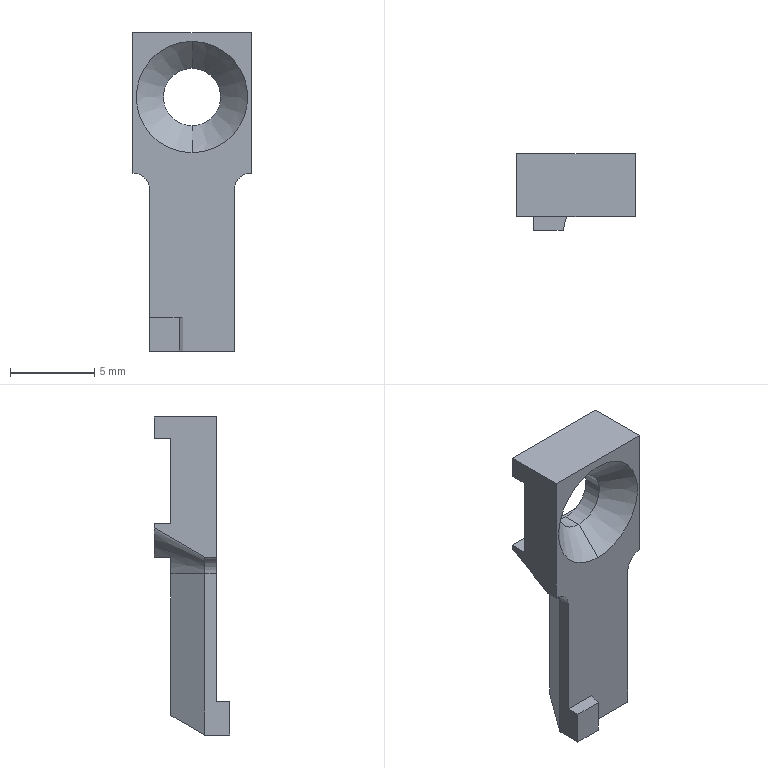Part | SolidWorks | features Cut 5, Chamfer 3, DelFace 1, Extrusion 1, Fillet 1, HoleWzd 1, MoveFace 1 | 1 solid | 26 faces | box 7 x 4.5 x 18.85 mm | volume 263.26 mm3 | plane 19 | cylinder 4 | cone 3 | commonest cylinder face diameters 2 x2 3.4 x2
STEP:
#1=CARTESIAN_POINT('',(0.,-2.1,7.325));
#2=VERTEX_POINT('',#1);
#3=CARTESIAN_POINT('',(0.,-2.1,3.925));
#4=VERTEX_POINT('',#3);
#5=CARTESIAN_POINT('',(0.,-2.1,5.625));
#6=DIRECTION('',(0.,-1.,0.));
#7=DIRECTION('',(0.,0.,-1.));
#8=AXIS2_PLACEMENT_3D('',#5,#6,#7);
#9=CIRCLE('',#8,1.7);
#10=EDGE_CURVE('',#2,#4,#9,.T.);
#11=ORIENTED_EDGE('',*,*,#10,.F.);
#12=CARTESIAN_POINT('',(0.,-3.7,8.925));
#13=VERTEX_POINT('',#12);
#14=CARTESIAN_POINT('',(0.,-3.7,8.925));
#15=DIRECTION('',(0.,-0.7071,0.7071));
#16=VECTOR('',#15,1000.);
#17=LINE('',#14,#16);
#18=EDGE_CURVE('',#2,#13,#17,.T.);
#19=ORIENTED_EDGE('',*,*,#18,.T.);
#20=CARTESIAN_POINT('',(0.,-3.7,2.325));
#21=VERTEX_POINT('',#20);
#22=CARTESIAN_POINT('',(0.,-3.7,5.625));
#23=DIRECTION('',(0.,-1.,0.));
#24=DIRECTION('',(0.,0.,-1.));
#25=AXIS2_PLACEMENT_3D('',#22,#23,#24);
#26=CIRCLE('',#25,3.3);
#27=EDGE_CURVE('',#13,#21,#26,.T.);
#28=ORIENTED_EDGE('',*,*,#27,.T.);
#29=CARTESIAN_POINT('',(0.,-3.7,2.325));
#30=DIRECTION('',(0.,-0.7071,-0.7071));
#31=VECTOR('',#30,1000.);
#32=LINE('',#29,#31);
#33=EDGE_CURVE('',#4,#21,#32,.T.);
#34=ORIENTED_EDGE('',*,*,#33,.F.);
#35=EDGE_LOOP('',(#11,#19,#28,#34));
#36=FACE_OUTER_BOUND('',#35,.T.);
#37=CARTESIAN_POINT('',(0.,-3.7,5.625));
#38=DIRECTION('',(0.,-1.,0.));
#39=DIRECTION('',(0.,0.,-1.));
#40=AXIS2_PLACEMENT_3D('',#37,#38,#39);
#41=CONICAL_SURFACE('',#40,3.3,0.7854);
#42=ADVANCED_FACE('',(#36),#41,.F.);
#43=CARTESIAN_POINT('',(0.,-1.,7.325));
#44=VERTEX_POINT('',#43);
#45=CARTESIAN_POINT('',(0.,-1.,3.925));
#46=VERTEX_POINT('',#45);
#47=CARTESIAN_POINT('',(0.,-1.,5.625));
#48=DIRECTION('',(0.,-1.,0.));
#49=DIRECTION('',(0.,0.,-1.));
#50=AXIS2_PLACEMENT_3D('',#47,#48,#49);
#51=CIRCLE('',#50,1.7);
#52=EDGE_CURVE('',#44,#46,#51,.T.);
#53=ORIENTED_EDGE('',*,*,#52,.F.);
#54=CARTESIAN_POINT('',(0.,-3.7,7.325));
#55=DIRECTION('',(0.,-1.,0.));
#56=VECTOR('',#55,1000.);
#57=LINE('',#54,#56);
#58=EDGE_CURVE('',#44,#2,#57,.T.);
#59=ORIENTED_EDGE('',*,*,#58,.T.);
#60=ORIENTED_EDGE('',*,*,#10,.T.);
#61=CARTESIAN_POINT('',(0.,-3.7,3.925));
#62=DIRECTION('',(0.,-1.,0.));
#63=VECTOR('',#62,1000.);
#64=LINE('',#61,#63);
#65=EDGE_CURVE('',#46,#4,#64,.T.);
#66=ORIENTED_EDGE('',*,*,#65,.F.);
#67=EDGE_LOOP('',(#53,#59,#60,#66));
#68=FACE_OUTER_BOUND('',#67,.T.);
#69=CARTESIAN_POINT('',(0.,-3.7,5.625));
#70=DIRECTION('',(0.,-1.,0.));
#71=DIRECTION('',(0.,0.,-1.));
#72=AXIS2_PLACEMENT_3D('',#69,#70,#71);
#73=CYLINDRICAL_SURFACE('',#72,1.7);
#74=ADVANCED_FACE('',(#68),#73,.F.);
#75=CARTESIAN_POINT('',(-3.5,-3.7,9.425));
#76=VERTEX_POINT('',#75);
#77=CARTESIAN_POINT('',(-3.5,0.,9.425));
#78=VERTEX_POINT('',#77);
#79=CARTESIAN_POINT('',(-3.5,-5.2,9.425));
#80=DIRECTION('',(0.,1.,0.));
#81=VECTOR('',#80,1000.);
#82=LINE('',#79,#81);
#83=EDGE_CURVE('',#76,#78,#82,.T.);
#84=ORIENTED_EDGE('',*,*,#83,.F.);
#85=CARTESIAN_POINT('',(3.5,-3.7,9.425));
#86=VERTEX_POINT('',#85);
#87=CARTESIAN_POINT('',(3.5,-3.7,9.425));
#88=DIRECTION('',(-1.,0.,0.));
#89=VECTOR('',#88,1000.);
#90=LINE('',#87,#89);
#91=EDGE_CURVE('',#86,#76,#90,.T.);
#92=ORIENTED_EDGE('',*,*,#91,.F.);
#93=CARTESIAN_POINT('',(3.5,0.,9.425));
#94=VERTEX_POINT('',#93);
#95=CARTESIAN_POINT('',(3.5,-5.2,9.425));
#96=DIRECTION('',(0.,1.,0.));
#97=VECTOR('',#96,1000.);
#98=LINE('',#95,#97);
#99=EDGE_CURVE('',#86,#94,#98,.T.);
#100=ORIENTED_EDGE('',*,*,#99,.T.);
#101=CARTESIAN_POINT('',(-3.5,0.,9.425));
#102=DIRECTION('',(1.,0.,0.));
#103=VECTOR('',#102,1000.);
#104=LINE('',#101,#103);
#105=EDGE_CURVE('',#78,#94,#104,.T.);
#106=ORIENTED_EDGE('',*,*,#105,.F.);
#107=EDGE_LOOP('',(#84,#92,#100,#106));
#108=FACE_OUTER_BOUND('',#107,.T.);
#109=CARTESIAN_POINT('',(-3.5,-5.2,9.425));
#110=DIRECTION('',(0.,0.,1.));
#111=DIRECTION('',(1.,0.,0.));
#112=AXIS2_PLACEMENT_3D('',#109,#110,#111);
#113=PLANE('',#112);
#114=ADVANCED_FACE('',(#108),#113,.T.);
#115=CARTESIAN_POINT('',(3.5,0.,8.125));
#116=VERTEX_POINT('',#115);
#117=CARTESIAN_POINT('',(3.5,0.,9.425));
#118=DIRECTION('',(0.,0.,-1.));
#119=VECTOR('',#118,1000.);
#120=LINE('',#117,#119);
#121=EDGE_CURVE('',#94,#116,#120,.T.);
#122=ORIENTED_EDGE('',*,*,#121,.T.);
#123=CARTESIAN_POINT('',(-3.5,0.,8.125));
#124=VERTEX_POINT('',#123);
#125=CARTESIAN_POINT('',(-3.5,0.,8.125));
#126=DIRECTION('',(1.,0.,0.));
#127=VECTOR('',#126,1000.);
#128=LINE('',#125,#127);
#129=EDGE_CURVE('',#124,#116,#128,.T.);
#130=ORIENTED_EDGE('',*,*,#129,.F.);
#131=CARTESIAN_POINT('',(-3.5,0.,9.425));
#132=DIRECTION('',(0.,0.,1.));
#133=VECTOR('',#132,1000.);
#134=LINE('',#131,#133);
#135=EDGE_CURVE('',#124,#78,#134,.T.);
#136=ORIENTED_EDGE('',*,*,#135,.T.);
#137=ORIENTED_EDGE('',*,*,#105,.T.);
#138=EDGE_LOOP('',(#122,#130,#136,#137));
#139=FACE_OUTER_BOUND('',#138,.T.);
#140=CARTESIAN_POINT('',(0.,0.,0.));
#141=DIRECTION('',(0.,-1.,0.));
#142=DIRECTION('',(0.,0.,-1.));
#143=AXIS2_PLACEMENT_3D('',#140,#141,#142);
#144=PLANE('',#143);
#145=ADVANCED_FACE('',(#139),#144,.F.);
#146=CARTESIAN_POINT('',(3.5,-3.7,1.125));
#147=VERTEX_POINT('',#146);
#148=CARTESIAN_POINT('',(3.5,-3.7,-7.425));
#149=DIRECTION('',(0.,0.,1.));
#150=VECTOR('',#149,1000.);
#151=LINE('',#148,#150);
#152=EDGE_CURVE('',#147,#86,#151,.T.);
#153=ORIENTED_EDGE('',*,*,#152,.F.);
#154=CARTESIAN_POINT('',(3.5,-1.,1.125));
#155=VERTEX_POINT('',#154);
#156=CARTESIAN_POINT('',(3.5,0.,1.125));
#157=DIRECTION('',(0.,-1.,0.));
#158=VECTOR('',#157,1000.);
#159=LINE('',#156,#158);
#160=EDGE_CURVE('',#155,#147,#159,.T.);
#161=ORIENTED_EDGE('',*,*,#160,.F.);
#162=CARTESIAN_POINT('',(3.5,0.,1.125));
#163=VERTEX_POINT('',#162);
#164=CARTESIAN_POINT('',(3.5,0.,1.125));
#165=DIRECTION('',(0.,-1.,0.));
#166=VECTOR('',#165,1000.);
#167=LINE('',#164,#166);
#168=EDGE_CURVE('',#163,#155,#167,.T.);
#169=ORIENTED_EDGE('',*,*,#168,.F.);
#170=CARTESIAN_POINT('',(3.5,0.,3.125));
#171=VERTEX_POINT('',#170);
#172=CARTESIAN_POINT('',(3.5,0.,9.425));
#173=DIRECTION('',(0.,0.,-1.));
#174=VECTOR('',#173,1000.);
#175=LINE('',#172,#174);
#176=EDGE_CURVE('',#171,#163,#175,.T.);
#177=ORIENTED_EDGE('',*,*,#176,.F.);
#178=CARTESIAN_POINT('',(3.5,-1.,3.125));
#179=VERTEX_POINT('',#178);
#180=CARTESIAN_POINT('',(3.5,0.,3.125));
#181=DIRECTION('',(0.,1.,0.));
#182=VECTOR('',#181,1000.);
#183=LINE('',#180,#182);
#184=EDGE_CURVE('',#179,#171,#183,.T.);
#185=ORIENTED_EDGE('',*,*,#184,.F.);
#186=CARTESIAN_POINT('',(3.5,-1.,8.125));
#187=VERTEX_POINT('',#186);
#188=CARTESIAN_POINT('',(3.5,-1.,8.125));
#189=DIRECTION('',(0.,0.,-1.));
#190=VECTOR('',#189,1000.);
#191=LINE('',#188,#190);
#192=EDGE_CURVE('',#187,#179,#191,.T.);
#193=ORIENTED_EDGE('',*,*,#192,.F.);
#194=CARTESIAN_POINT('',(3.5,0.,8.125));
#195=DIRECTION('',(0.,-1.,0.));
#196=VECTOR('',#195,1000.);
#197=LINE('',#194,#196);
#198=EDGE_CURVE('',#116,#187,#197,.T.);
#199=ORIENTED_EDGE('',*,*,#198,.F.);
#200=ORIENTED_EDGE('',*,*,#121,.F.);
#201=ORIENTED_EDGE('',*,*,#99,.F.);
#202=EDGE_LOOP('',(#153,#161,#169,#177,#185,#193,#199,#200,#201));
#203=FACE_OUTER_BOUND('',#202,.T.);
#204=CARTESIAN_POINT('',(3.5,-5.2,9.425));
#205=DIRECTION('',(1.,0.,0.));
#206=DIRECTION('',(0.,0.,-1.));
#207=AXIS2_PLACEMENT_3D('',#204,#205,#206);
#208=PLANE('',#207);
#209=ADVANCED_FACE('',(#203),#208,.T.);
#210=CARTESIAN_POINT('',(-3.5,0.,2.857));
#211=VERTEX_POINT('',#210);
#212=CARTESIAN_POINT('',(-3.5,0.,3.125));
#213=VERTEX_POINT('',#212);
#214=CARTESIAN_POINT('',(-3.5,0.,9.425));
#215=DIRECTION('',(0.,0.,1.));
#216=VECTOR('',#215,1000.);
#217=LINE('',#214,#216);
#218=EDGE_CURVE('',#211,#213,#217,.T.);
#219=ORIENTED_EDGE('',*,*,#218,.F.);
#220=CARTESIAN_POINT('',(-3.5,-3.,1.125));
#221=VERTEX_POINT('',#220);
#222=CARTESIAN_POINT('',(-3.5,-4.732,0.125));
#223=DIRECTION('',(0.,-0.866,-0.5));
#224=VECTOR('',#223,1000.);
#225=LINE('',#222,#224);
#226=EDGE_CURVE('',#211,#221,#225,.T.);
#227=ORIENTED_EDGE('',*,*,#226,.T.);
#228=CARTESIAN_POINT('',(-3.5,-3.7,1.125));
#229=VERTEX_POINT('',#228);
#230=CARTESIAN_POINT('',(-3.5,0.,1.125));
#231=DIRECTION('',(0.,-1.,0.));
#232=VECTOR('',#231,1000.);
#233=LINE('',#230,#232);
#234=EDGE_CURVE('',#221,#229,#233,.T.);
#235=ORIENTED_EDGE('',*,*,#234,.T.);
#236=CARTESIAN_POINT('',(-3.5,-3.7,9.425));
#237=DIRECTION('',(0.,0.,-1.));
#238=VECTOR('',#237,1000.);
#239=LINE('',#236,#238);
#240=EDGE_CURVE('',#76,#229,#239,.T.);
#241=ORIENTED_EDGE('',*,*,#240,.F.);
#242=ORIENTED_EDGE('',*,*,#83,.T.);
#243=ORIENTED_EDGE('',*,*,#135,.F.);
#244=CARTESIAN_POINT('',(-3.5,-1.,8.125));
#245=VERTEX_POINT('',#244);
#246=CARTESIAN_POINT('',(-3.5,0.,8.125));
#247=DIRECTION('',(0.,-1.,0.));
#248=VECTOR('',#247,1000.);
#249=LINE('',#246,#248);
#250=EDGE_CURVE('',#124,#245,#249,.T.);
#251=ORIENTED_EDGE('',*,*,#250,.T.);
#252=CARTESIAN_POINT('',(-3.5,-1.,3.125));
#253=VERTEX_POINT('',#252);
#254=CARTESIAN_POINT('',(-3.5,-1.,8.125));
#255=DIRECTION('',(0.,0.,-1.));
#256=VECTOR('',#255,1000.);
#257=LINE('',#254,#256);
#258=EDGE_CURVE('',#245,#253,#257,.T.);
#259=ORIENTED_EDGE('',*,*,#258,.T.);
#260=CARTESIAN_POINT('',(-3.5,0.,3.125));
#261=DIRECTION('',(0.,1.,0.));
#262=VECTOR('',#261,1000.);
#263=LINE('',#260,#262);
#264=EDGE_CURVE('',#253,#213,#263,.T.);
#265=ORIENTED_EDGE('',*,*,#264,.T.);
#266=EDGE_LOOP('',(#219,#227,#235,#241,#242,#243,#251,#259,#265));
#267=FACE_OUTER_BOUND('',#266,.T.);
#268=CARTESIAN_POINT('',(-3.5,-5.2,9.425));
#269=DIRECTION('',(-1.,0.,0.));
#270=DIRECTION('',(0.,0.,1.));
#271=AXIS2_PLACEMENT_3D('',#268,#269,#270);
#272=PLANE('',#271);
#273=ADVANCED_FACE('',(#267),#272,.T.);
#274=CARTESIAN_POINT('',(-2.5,-4.5,-9.425));
#275=VERTEX_POINT('',#274);
#276=CARTESIAN_POINT('',(-2.5,-3.,-9.425));
#277=VERTEX_POINT('',#276);
#278=CARTESIAN_POINT('',(-2.5,-5.2,-9.425));
#279=DIRECTION('',(0.,1.,0.));
#280=VECTOR('',#279,1000.);
#281=LINE('',#278,#280);
#282=EDGE_CURVE('',#275,#277,#281,.T.);
#283=ORIENTED_EDGE('',*,*,#282,.T.);
#284=CARTESIAN_POINT('',(2.5,-3.,-9.425));
#285=VERTEX_POINT('',#284);
#286=CARTESIAN_POINT('',(2.5,-3.,-9.425));
#287=DIRECTION('',(1.,0.,0.));
#288=VECTOR('',#287,1000.);
#289=LINE('',#286,#288);
#290=EDGE_CURVE('',#277,#285,#289,.T.);
#291=ORIENTED_EDGE('',*,*,#290,.T.);
#292=CARTESIAN_POINT('',(2.5,-3.7,-9.425));
#293=VERTEX_POINT('',#292);
#294=CARTESIAN_POINT('',(2.5,-5.2,-9.425));
#295=DIRECTION('',(0.,1.,0.));
#296=VECTOR('',#295,1000.);
#297=LINE('',#294,#296);
#298=EDGE_CURVE('',#293,#285,#297,.T.);
#299=ORIENTED_EDGE('',*,*,#298,.F.);
#300=CARTESIAN_POINT('',(-0.5536,-3.7,-9.425));
#301=VERTEX_POINT('',#300);
#302=CARTESIAN_POINT('',(-0.5,-3.7,-9.425));
#303=DIRECTION('',(1.,0.,0.));
#304=VECTOR('',#303,1000.);
#305=LINE('',#302,#304);
#306=EDGE_CURVE('',#301,#293,#305,.T.);
#307=ORIENTED_EDGE('',*,*,#306,.F.);
#308=CARTESIAN_POINT('',(-0.7679,-4.5,-9.425));
#309=VERTEX_POINT('',#308);
#310=CARTESIAN_POINT('',(-0.951,-5.183,-9.425));
#311=DIRECTION('',(-0.2588,-0.9659,0.));
#312=VECTOR('',#311,1000.);
#313=LINE('',#310,#312);
#314=EDGE_CURVE('',#301,#309,#313,.T.);
#315=ORIENTED_EDGE('',*,*,#314,.T.);
#316=CARTESIAN_POINT('',(-3.5,-4.5,-9.425));
#317=DIRECTION('',(-1.,0.,0.));
#318=VECTOR('',#317,1000.);
#319=LINE('',#316,#318);
#320=EDGE_CURVE('',#309,#275,#319,.T.);
#321=ORIENTED_EDGE('',*,*,#320,.T.);
#322=EDGE_LOOP('',(#283,#291,#299,#307,#315,#321));
#323=FACE_OUTER_BOUND('',#322,.T.);
#324=CARTESIAN_POINT('',(-3.5,-5.2,-9.425));
#325=DIRECTION('',(0.,0.,-1.));
#326=DIRECTION('',(-1.,0.,0.));
#327=AXIS2_PLACEMENT_3D('',#324,#325,#326);
#328=PLANE('',#327);
#329=ADVANCED_FACE('',(#323),#328,.T.);
#330=ORIENTED_EDGE('',*,*,#320,.F.);
#331=CARTESIAN_POINT('',(-0.7679,-4.5,-7.425));
#332=VERTEX_POINT('',#331);
#333=CARTESIAN_POINT('',(-0.7679,-4.5,-8.085));
#334=DIRECTION('',(0.,0.,1.));
#335=VECTOR('',#334,1000.);
#336=LINE('',#333,#335);
#337=EDGE_CURVE('',#309,#332,#336,.T.);
#338=ORIENTED_EDGE('',*,*,#337,.T.);
#339=CARTESIAN_POINT('',(-2.5,-4.5,-7.425));
#340=VERTEX_POINT('',#339);
#341=CARTESIAN_POINT('',(-3.5,-4.5,-7.425));
#342=DIRECTION('',(1.,0.,0.));
#343=VECTOR('',#342,1000.);
#344=LINE('',#341,#343);
#345=EDGE_CURVE('',#340,#332,#344,.T.);
#346=ORIENTED_EDGE('',*,*,#345,.F.);
#347=CARTESIAN_POINT('',(-2.5,-4.5,-9.425));
#348=DIRECTION('',(0.,0.,-1.));
#349=VECTOR('',#348,1000.);
#350=LINE('',#347,#349);
#351=EDGE_CURVE('',#340,#275,#350,.T.);
#352=ORIENTED_EDGE('',*,*,#351,.T.);
#353=EDGE_LOOP('',(#330,#338,#346,#352));
#354=FACE_OUTER_BOUND('',#353,.T.);
#355=CARTESIAN_POINT('',(0.,-4.5,0.));
#356=DIRECTION('',(0.,-1.,0.));
#357=DIRECTION('',(0.,0.,-1.));
#358=AXIS2_PLACEMENT_3D('',#355,#356,#357);
#359=PLANE('',#358);
#360=ADVANCED_FACE('',(#354),#359,.T.);
#361=CARTESIAN_POINT('',(-0.9575,0.,1.125));
#362=VERTEX_POINT('',#361);
#363=CARTESIAN_POINT('',(-3.5,0.,1.125));
#364=DIRECTION('',(1.,0.,0.));
#365=VECTOR('',#364,1000.);
#366=LINE('',#363,#365);
#367=EDGE_CURVE('',#362,#163,#366,.T.);
#368=ORIENTED_EDGE('',*,*,#367,.F.);
#369=CARTESIAN_POINT('',(-3.5,0.,0.125));
#370=DIRECTION('',(0.,-1.,0.));
#371=DIRECTION('',(0.,0.,-1.));
#372=AXIS2_PLACEMENT_3D('',#369,#370,#371);
#373=CIRCLE('',#372,2.732);
#374=EDGE_CURVE('',#362,#211,#373,.T.);
#375=ORIENTED_EDGE('',*,*,#374,.T.);
#376=ORIENTED_EDGE('',*,*,#218,.T.);
#377=CARTESIAN_POINT('',(-3.5,0.,3.125));
#378=DIRECTION('',(1.,0.,0.));
#379=VECTOR('',#378,1000.);
#380=LINE('',#377,#379);
#381=EDGE_CURVE('',#213,#171,#380,.T.);
#382=ORIENTED_EDGE('',*,*,#381,.T.);
#383=ORIENTED_EDGE('',*,*,#176,.T.);
#384=EDGE_LOOP('',(#368,#375,#376,#382,#383));
#385=FACE_OUTER_BOUND('',#384,.T.);
#386=CARTESIAN_POINT('',(0.,0.,0.));
#387=DIRECTION('',(0.,-1.,0.));
#388=DIRECTION('',(0.,0.,-1.));
#389=AXIS2_PLACEMENT_3D('',#386,#387,#388);
#390=PLANE('',#389);
#391=ADVANCED_FACE('',(#385),#390,.F.);
#392=ORIENTED_EDGE('',*,*,#198,.T.);
#393=CARTESIAN_POINT('',(-3.5,-1.,8.125));
#394=DIRECTION('',(1.,0.,0.));
#395=VECTOR('',#394,1000.);
#396=LINE('',#393,#395);
#397=EDGE_CURVE('',#245,#187,#396,.T.);
#398=ORIENTED_EDGE('',*,*,#397,.F.);
#399=ORIENTED_EDGE('',*,*,#250,.F.);
#400=ORIENTED_EDGE('',*,*,#129,.T.);
#401=EDGE_LOOP('',(#392,#398,#399,#400));
#402=FACE_OUTER_BOUND('',#401,.T.);
#403=CARTESIAN_POINT('',(-3.5,0.,8.125));
#404=DIRECTION('',(0.,0.,1.));
#405=DIRECTION('',(1.,0.,0.));
#406=AXIS2_PLACEMENT_3D('',#403,#404,#405);
#407=PLANE('',#406);
#408=ADVANCED_FACE('',(#402),#407,.F.);
#409=ORIENTED_EDGE('',*,*,#184,.T.);
#410=ORIENTED_EDGE('',*,*,#381,.F.);
#411=ORIENTED_EDGE('',*,*,#264,.F.);
#412=CARTESIAN_POINT('',(-3.5,-1.,3.125));
#413=DIRECTION('',(1.,0.,0.));
#414=VECTOR('',#413,1000.);
#415=LINE('',#412,#414);
#416=EDGE_CURVE('',#253,#179,#415,.T.);
#417=ORIENTED_EDGE('',*,*,#416,.T.);
#418=EDGE_LOOP('',(#409,#410,#411,#417));
#419=FACE_OUTER_BOUND('',#418,.T.);
#420=CARTESIAN_POINT('',(-3.5,0.,3.125));
#421=DIRECTION('',(0.,0.,-1.));
#422=DIRECTION('',(-1.,0.,0.));
#423=AXIS2_PLACEMENT_3D('',#420,#421,#422);
#424=PLANE('',#423);
#425=ADVANCED_FACE('',(#419),#424,.F.);
#426=CARTESIAN_POINT('',(0.,-1.,5.625));
#427=DIRECTION('',(0.,-1.,0.));
#428=DIRECTION('',(0.,0.,-1.));
#429=AXIS2_PLACEMENT_3D('',#426,#427,#428);
#430=CIRCLE('',#429,1.7);
#431=EDGE_CURVE('',#46,#44,#430,.T.);
#432=ORIENTED_EDGE('',*,*,#431,.T.);
#433=ORIENTED_EDGE('',*,*,#52,.T.);
#434=EDGE_LOOP('',(#432,#433));
#435=FACE_BOUND('',#434,.T.);
#436=ORIENTED_EDGE('',*,*,#192,.T.);
#437=ORIENTED_EDGE('',*,*,#416,.F.);
#438=ORIENTED_EDGE('',*,*,#258,.F.);
#439=ORIENTED_EDGE('',*,*,#397,.T.);
#440=EDGE_LOOP('',(#436,#437,#438,#439));
#441=FACE_OUTER_BOUND('',#440,.T.);
#442=CARTESIAN_POINT('',(-3.5,-1.,8.125));
#443=DIRECTION('',(0.,-1.,0.));
#444=DIRECTION('',(0.,0.,-1.));
#445=AXIS2_PLACEMENT_3D('',#442,#443,#444);
#446=PLANE('',#445);
#447=ADVANCED_FACE('',(#435,#441),#446,.F.);
#448=CARTESIAN_POINT('',(-1.591,-1.,1.125));
#449=VERTEX_POINT('',#448);
#450=CARTESIAN_POINT('',(-3.5,-1.,1.125));
#451=DIRECTION('',(1.,0.,0.));
#452=VECTOR('',#451,1000.);
#453=LINE('',#450,#452);
#454=EDGE_CURVE('',#449,#155,#453,.T.);
#455=ORIENTED_EDGE('',*,*,#454,.F.);
#456=CARTESIAN_POINT('',(-1.591,-1.,1.125));
#457=CARTESIAN_POINT('',(-1.376,-0.6693,1.125));
#458=CARTESIAN_POINT('',(-1.166,-0.3354,1.125));
#459=CARTESIAN_POINT('',(-0.9575,0.,1.125));
#460=B_SPLINE_CURVE_WITH_KNOTS('',3,(#456,#457,#458,#459),.UNSPECIFIED.,.F.,.F.,(4,4),(0.,0.001184),.UNSPECIFIED.);
#461=EDGE_CURVE('',#449,#362,#460,.T.);
#462=ORIENTED_EDGE('',*,*,#461,.T.);
#463=ORIENTED_EDGE('',*,*,#367,.T.);
#464=ORIENTED_EDGE('',*,*,#168,.T.);
#465=EDGE_LOOP('',(#455,#462,#463,#464));
#466=FACE_OUTER_BOUND('',#465,.T.);
#467=CARTESIAN_POINT('',(-3.5,0.,1.125));
#468=DIRECTION('',(0.,0.,1.));
#469=DIRECTION('',(0.,-1.,0.));
#470=AXIS2_PLACEMENT_3D('',#467,#468,#469);
#471=PLANE('',#470);
#472=ADVANCED_FACE('',(#466),#471,.F.);
#473=CARTESIAN_POINT('',(-1.345,-1.,-8.27));
#474=VERTEX_POINT('',#473);
#475=CARTESIAN_POINT('',(-1.345,-1.,0.125));
#476=VERTEX_POINT('',#475);
#477=CARTESIAN_POINT('',(-1.345,-1.,1.125));
#478=DIRECTION('',(0.,0.,1.));
#479=VECTOR('',#478,1000.);
#480=LINE('',#477,#479);
#481=EDGE_CURVE('',#474,#476,#480,.T.);
#482=ORIENTED_EDGE('',*,*,#481,.T.);
#483=CARTESIAN_POINT('',(-3.5,-1.,0.125));
#484=DIRECTION('',(0.,-1.,0.));
#485=DIRECTION('',(0.,0.,-1.));
#486=AXIS2_PLACEMENT_3D('',#483,#484,#485);
#487=CIRCLE('',#486,2.155);
#488=EDGE_CURVE('',#476,#449,#487,.T.);
#489=ORIENTED_EDGE('',*,*,#488,.T.);
#490=ORIENTED_EDGE('',*,*,#454,.T.);
#491=CARTESIAN_POINT('',(2.5,-1.,0.125));
#492=VERTEX_POINT('',#491);
#493=CARTESIAN_POINT('',(3.5,-1.,0.125));
#494=DIRECTION('',(0.,-1.,0.));
#495=DIRECTION('',(0.,0.,-1.));
#496=AXIS2_PLACEMENT_3D('',#493,#494,#495);
#497=CIRCLE('',#496,1.);
#498=EDGE_CURVE('',#155,#492,#497,.T.);
#499=ORIENTED_EDGE('',*,*,#498,.T.);
#500=CARTESIAN_POINT('',(2.5,-1.,-8.27));
#501=VERTEX_POINT('',#500);
#502=CARTESIAN_POINT('',(2.5,-1.,-9.425));
#503=DIRECTION('',(0.,0.,1.));
#504=VECTOR('',#503,1000.);
#505=LINE('',#502,#504);
#506=EDGE_CURVE('',#501,#492,#505,.T.);
#507=ORIENTED_EDGE('',*,*,#506,.F.);
#508=CARTESIAN_POINT('',(-2.5,-1.,-8.27));
#509=DIRECTION('',(-1.,0.,0.));
#510=VECTOR('',#509,1000.);
#511=LINE('',#508,#510);
#512=EDGE_CURVE('',#501,#474,#511,.T.);
#513=ORIENTED_EDGE('',*,*,#512,.T.);
#514=EDGE_LOOP('',(#482,#489,#490,#499,#507,#513));
#515=FACE_OUTER_BOUND('',#514,.T.);
#516=CARTESIAN_POINT('',(-3.5,-1.,1.125));
#517=DIRECTION('',(0.,-1.,0.));
#518=DIRECTION('',(0.,0.,-1.));
#519=AXIS2_PLACEMENT_3D('',#516,#517,#518);
#520=PLANE('',#519);
#521=ADVANCED_FACE('',(#515),#520,.F.);
#522=CARTESIAN_POINT('',(-0.5536,-3.7,-7.425));
#523=VERTEX_POINT('',#522);
#524=CARTESIAN_POINT('',(-0.5,-3.5,-7.425));
#525=DIRECTION('',(0.2588,0.9659,0.));
#526=VECTOR('',#525,1000.);
#527=LINE('',#524,#526);
#528=EDGE_CURVE('',#332,#523,#527,.T.);
#529=ORIENTED_EDGE('',*,*,#528,.T.);
#530=CARTESIAN_POINT('',(-2.5,-3.7,-7.425));
#531=VERTEX_POINT('',#530);
#532=CARTESIAN_POINT('',(0.48,-3.7,-7.425));
#533=DIRECTION('',(1.,0.,0.));
#534=VECTOR('',#533,1000.);
#535=LINE('',#532,#534);
#536=EDGE_CURVE('',#531,#523,#535,.T.);
#537=ORIENTED_EDGE('',*,*,#536,.F.);
#538=CARTESIAN_POINT('',(-2.5,-3.7,-7.425));
#539=DIRECTION('',(0.,-1.,0.));
#540=VECTOR('',#539,1000.);
#541=LINE('',#538,#540);
#542=EDGE_CURVE('',#531,#340,#541,.T.);
#543=ORIENTED_EDGE('',*,*,#542,.T.);
#544=ORIENTED_EDGE('',*,*,#345,.T.);
#545=EDGE_LOOP('',(#529,#537,#543,#544));
#546=FACE_OUTER_BOUND('',#545,.T.);
#547=CARTESIAN_POINT('',(0.48,-3.7,-7.425));
#548=DIRECTION('',(0.,0.,-1.));
#549=DIRECTION('',(-1.,0.,0.));
#550=AXIS2_PLACEMENT_3D('',#547,#548,#549);
#551=PLANE('',#550);
#552=ADVANCED_FACE('',(#546),#551,.F.);
#553=CARTESIAN_POINT('',(0.,-3.7,5.625));
#554=DIRECTION('',(0.,-1.,0.));
#555=DIRECTION('',(0.,0.,-1.));
#556=AXIS2_PLACEMENT_3D('',#553,#554,#555);
#557=CIRCLE('',#556,3.3);
#558=EDGE_CURVE('',#21,#13,#557,.T.);
#559=ORIENTED_EDGE('',*,*,#558,.F.);
#560=ORIENTED_EDGE('',*,*,#27,.F.);
#561=EDGE_LOOP('',(#559,#560));
#562=FACE_BOUND('',#561,.T.);
#563=CARTESIAN_POINT('',(2.5,-3.7,0.125));
#564=VERTEX_POINT('',#563);
#565=CARTESIAN_POINT('',(2.5,-3.7,-6.345));
#566=DIRECTION('',(0.,0.,-1.));
#567=VECTOR('',#566,1000.);
#568=LINE('',#565,#567);
#569=EDGE_CURVE('',#564,#293,#568,.T.);
#570=ORIENTED_EDGE('',*,*,#569,.F.);
#571=CARTESIAN_POINT('',(3.5,-3.7,0.125));
#572=DIRECTION('',(0.,1.,0.));
#573=DIRECTION('',(0.,0.,-1.));
#574=AXIS2_PLACEMENT_3D('',#571,#572,#573);
#575=CIRCLE('',#574,1.);
#576=EDGE_CURVE('',#564,#147,#575,.T.);
#577=ORIENTED_EDGE('',*,*,#576,.T.);
#578=ORIENTED_EDGE('',*,*,#152,.T.);
#579=ORIENTED_EDGE('',*,*,#91,.T.);
#580=ORIENTED_EDGE('',*,*,#240,.T.);
#581=CARTESIAN_POINT('',(-2.5,-3.7,0.125));
#582=VERTEX_POINT('',#581);
#583=CARTESIAN_POINT('',(-3.5,-3.7,0.125));
#584=DIRECTION('',(0.,1.,0.));
#585=DIRECTION('',(0.,0.,-1.));
#586=AXIS2_PLACEMENT_3D('',#583,#584,#585);
#587=CIRCLE('',#586,1.);
#588=EDGE_CURVE('',#229,#582,#587,.T.);
#589=ORIENTED_EDGE('',*,*,#588,.T.);
#590=CARTESIAN_POINT('',(-2.5,-3.7,-6.345));
#591=DIRECTION('',(0.,0.,1.));
#592=VECTOR('',#591,1000.);
#593=LINE('',#590,#592);
#594=EDGE_CURVE('',#531,#582,#593,.T.);
#595=ORIENTED_EDGE('',*,*,#594,.F.);
#596=ORIENTED_EDGE('',*,*,#536,.T.);
#597=CARTESIAN_POINT('',(-0.5536,-3.7,9.425));
#598=DIRECTION('',(0.,0.,-1.));
#599=VECTOR('',#598,1000.);
#600=LINE('',#597,#599);
#601=EDGE_CURVE('',#523,#301,#600,.T.);
#602=ORIENTED_EDGE('',*,*,#601,.T.);
#603=ORIENTED_EDGE('',*,*,#306,.T.);
#604=EDGE_LOOP('',(#570,#577,#578,#579,#580,#589,#595,#596,#602,#603));
#605=FACE_OUTER_BOUND('',#604,.T.);
#606=CARTESIAN_POINT('',(-0.96,-3.7,-6.345));
#607=DIRECTION('',(0.,-1.,0.));
#608=DIRECTION('',(0.,0.,-1.));
#609=AXIS2_PLACEMENT_3D('',#606,#607,#608);
#610=PLANE('',#609);
#611=ADVANCED_FACE('',(#562,#605),#610,.T.);
#612=CARTESIAN_POINT('',(-2.5,-3.,0.125));
#613=VERTEX_POINT('',#612);
#614=CARTESIAN_POINT('',(-2.5,-1.,0.125));
#615=DIRECTION('',(0.,1.,0.));
#616=VECTOR('',#615,1000.);
#617=LINE('',#614,#616);
#618=EDGE_CURVE('',#582,#613,#617,.T.);
#619=ORIENTED_EDGE('',*,*,#618,.T.);
#620=CARTESIAN_POINT('',(-2.5,-3.,-9.425));
#621=DIRECTION('',(0.,0.,-1.));
#622=VECTOR('',#621,1000.);
#623=LINE('',#620,#622);
#624=EDGE_CURVE('',#613,#277,#623,.T.);
#625=ORIENTED_EDGE('',*,*,#624,.T.);
#626=ORIENTED_EDGE('',*,*,#282,.F.);
#627=ORIENTED_EDGE('',*,*,#351,.F.);
#628=ORIENTED_EDGE('',*,*,#542,.F.);
#629=ORIENTED_EDGE('',*,*,#594,.T.);
#630=EDGE_LOOP('',(#619,#625,#626,#627,#628,#629));
#631=FACE_OUTER_BOUND('',#630,.T.);
#632=CARTESIAN_POINT('',(-2.5,-5.2,-9.425));
#633=DIRECTION('',(1.,0.,0.));
#634=DIRECTION('',(0.,0.,-1.));
#635=AXIS2_PLACEMENT_3D('',#632,#633,#634);
#636=PLANE('',#635);
#637=ADVANCED_FACE('',(#631),#636,.F.);
#638=ORIENTED_EDGE('',*,*,#298,.T.);
#639=CARTESIAN_POINT('',(2.5,-3.,-9.425));
#640=DIRECTION('',(0.,0.866,0.5));
#641=VECTOR('',#640,1000.);
#642=LINE('',#639,#641);
#643=EDGE_CURVE('',#285,#501,#642,.T.);
#644=ORIENTED_EDGE('',*,*,#643,.T.);
#645=ORIENTED_EDGE('',*,*,#506,.T.);
#646=CARTESIAN_POINT('',(2.5,-3.7,0.125));
#647=DIRECTION('',(0.,-1.,0.));
#648=VECTOR('',#647,1000.);
#649=LINE('',#646,#648);
#650=EDGE_CURVE('',#492,#564,#649,.T.);
#651=ORIENTED_EDGE('',*,*,#650,.T.);
#652=ORIENTED_EDGE('',*,*,#569,.T.);
#653=EDGE_LOOP('',(#638,#644,#645,#651,#652));
#654=FACE_OUTER_BOUND('',#653,.T.);
#655=CARTESIAN_POINT('',(2.5,-5.2,-9.425));
#656=DIRECTION('',(-1.,0.,0.));
#657=DIRECTION('',(0.,0.,1.));
#658=AXIS2_PLACEMENT_3D('',#655,#656,#657);
#659=PLANE('',#658);
#660=ADVANCED_FACE('',(#654),#659,.F.);
#661=ORIENTED_EDGE('',*,*,#58,.F.);
#662=ORIENTED_EDGE('',*,*,#431,.F.);
#663=ORIENTED_EDGE('',*,*,#65,.T.);
#664=CARTESIAN_POINT('',(0.,-2.1,5.625));
#665=DIRECTION('',(0.,-1.,0.));
#666=DIRECTION('',(0.,0.,-1.));
#667=AXIS2_PLACEMENT_3D('',#664,#665,#666);
#668=CIRCLE('',#667,1.7);
#669=EDGE_CURVE('',#4,#2,#668,.T.);
#670=ORIENTED_EDGE('',*,*,#669,.T.);
#671=EDGE_LOOP('',(#661,#662,#663,#670));
#672=FACE_OUTER_BOUND('',#671,.T.);
#673=CARTESIAN_POINT('',(0.,-3.7,5.625));
#674=DIRECTION('',(0.,-1.,0.));
#675=DIRECTION('',(0.,0.,-1.));
#676=AXIS2_PLACEMENT_3D('',#673,#674,#675);
#677=CYLINDRICAL_SURFACE('',#676,1.7);
#678=ADVANCED_FACE('',(#672),#677,.F.);
#679=ORIENTED_EDGE('',*,*,#18,.F.);
#680=ORIENTED_EDGE('',*,*,#669,.F.);
#681=ORIENTED_EDGE('',*,*,#33,.T.);
#682=ORIENTED_EDGE('',*,*,#558,.T.);
#683=EDGE_LOOP('',(#679,#680,#681,#682));
#684=FACE_OUTER_BOUND('',#683,.T.);
#685=CARTESIAN_POINT('',(0.,-3.7,5.625));
#686=DIRECTION('',(0.,-1.,0.));
#687=DIRECTION('',(0.,0.,-1.));
#688=AXIS2_PLACEMENT_3D('',#685,#686,#687);
#689=CONICAL_SURFACE('',#688,3.3,0.7854);
#690=ADVANCED_FACE('',(#684),#689,.F.);
#691=ORIENTED_EDGE('',*,*,#234,.F.);
#692=CARTESIAN_POINT('',(-3.5,-3.,0.125));
#693=DIRECTION('',(0.,1.,0.));
#694=DIRECTION('',(0.,0.,-1.));
#695=AXIS2_PLACEMENT_3D('',#692,#693,#694);
#696=CIRCLE('',#695,1.);
#697=EDGE_CURVE('',#221,#613,#696,.T.);
#698=ORIENTED_EDGE('',*,*,#697,.T.);
#699=ORIENTED_EDGE('',*,*,#618,.F.);
#700=ORIENTED_EDGE('',*,*,#588,.F.);
#701=EDGE_LOOP('',(#691,#698,#699,#700));
#702=FACE_OUTER_BOUND('',#701,.T.);
#703=CARTESIAN_POINT('',(-3.5,-5.2,0.125));
#704=DIRECTION('',(0.,-1.,0.));
#705=DIRECTION('',(0.,0.,-1.));
#706=AXIS2_PLACEMENT_3D('',#703,#704,#705);
#707=CYLINDRICAL_SURFACE('',#706,1.);
#708=ADVANCED_FACE('',(#702),#707,.F.);
#709=ORIENTED_EDGE('',*,*,#576,.F.);
#710=ORIENTED_EDGE('',*,*,#650,.F.);
#711=ORIENTED_EDGE('',*,*,#498,.F.);
#712=ORIENTED_EDGE('',*,*,#160,.T.);
#713=EDGE_LOOP('',(#709,#710,#711,#712));
#714=FACE_OUTER_BOUND('',#713,.T.);
#715=CARTESIAN_POINT('',(3.5,0.,0.125));
#716=DIRECTION('',(0.,-1.,0.));
#717=DIRECTION('',(0.,0.,-1.));
#718=AXIS2_PLACEMENT_3D('',#715,#716,#717);
#719=CYLINDRICAL_SURFACE('',#718,1.);
#720=ADVANCED_FACE('',(#714),#719,.F.);
#721=ORIENTED_EDGE('',*,*,#601,.F.);
#722=ORIENTED_EDGE('',*,*,#528,.F.);
#723=ORIENTED_EDGE('',*,*,#337,.F.);
#724=ORIENTED_EDGE('',*,*,#314,.F.);
#725=EDGE_LOOP('',(#721,#722,#723,#724));
#726=FACE_OUTER_BOUND('',#725,.T.);
#727=CARTESIAN_POINT('',(-0.5,-3.5,9.425));
#728=DIRECTION('',(0.9659,-0.2588,0.));
#729=DIRECTION('',(0.,0.,1.));
#730=AXIS2_PLACEMENT_3D('',#727,#728,#729);
#731=PLANE('',#730);
#732=ADVANCED_FACE('',(#726),#731,.T.);
#733=ORIENTED_EDGE('',*,*,#643,.F.);
#734=ORIENTED_EDGE('',*,*,#290,.F.);
#735=CARTESIAN_POINT('',(-2.5,-3.,-9.425));
#736=DIRECTION('',(-0.4472,-0.7746,-0.4472));
#737=VECTOR('',#736,1000.);
#738=LINE('',#735,#737);
#739=EDGE_CURVE('',#474,#277,#738,.T.);
#740=ORIENTED_EDGE('',*,*,#739,.F.);
#741=ORIENTED_EDGE('',*,*,#512,.F.);
#742=EDGE_LOOP('',(#733,#734,#740,#741));
#743=FACE_OUTER_BOUND('',#742,.T.);
#744=CARTESIAN_POINT('',(-3.5,-3.,-9.425));
#745=DIRECTION('',(0.,0.5,-0.866));
#746=DIRECTION('',(-1.,0.,0.));
#747=AXIS2_PLACEMENT_3D('',#744,#745,#746);
#748=PLANE('',#747);
#749=ADVANCED_FACE('',(#743),#748,.T.);
#750=ORIENTED_EDGE('',*,*,#739,.T.);
#751=ORIENTED_EDGE('',*,*,#624,.F.);
#752=CARTESIAN_POINT('',(-1.345,-1.,0.125));
#753=DIRECTION('',(-0.5,-0.866,0.));
#754=VECTOR('',#753,1000.);
#755=LINE('',#752,#754);
#756=EDGE_CURVE('',#476,#613,#755,.T.);
#757=ORIENTED_EDGE('',*,*,#756,.F.);
#758=ORIENTED_EDGE('',*,*,#481,.F.);
#759=EDGE_LOOP('',(#750,#751,#757,#758));
#760=FACE_OUTER_BOUND('',#759,.T.);
#761=CARTESIAN_POINT('',(-2.5,-3.,-9.425));
#762=DIRECTION('',(0.866,-0.5,0.));
#763=DIRECTION('',(0.,0.,-1.));
#764=AXIS2_PLACEMENT_3D('',#761,#762,#763);
#765=PLANE('',#764);
#766=ADVANCED_FACE('',(#760),#765,.F.);
#767=ORIENTED_EDGE('',*,*,#756,.T.);
#768=ORIENTED_EDGE('',*,*,#697,.F.);
#769=ORIENTED_EDGE('',*,*,#226,.F.);
#770=ORIENTED_EDGE('',*,*,#374,.F.);
#771=ORIENTED_EDGE('',*,*,#461,.F.);
#772=ORIENTED_EDGE('',*,*,#488,.F.);
#773=EDGE_LOOP('',(#767,#768,#769,#770,#771,#772));
#774=FACE_OUTER_BOUND('',#773,.T.);
#775=CARTESIAN_POINT('',(-3.5,-1.,0.125));
#776=DIRECTION('',(0.,1.,0.));
#777=DIRECTION('',(0.,0.,1.));
#778=AXIS2_PLACEMENT_3D('',#775,#776,#777);
#779=CONICAL_SURFACE('',#778,2.155,0.5236);
#780=ADVANCED_FACE('',(#774),#779,.F.);
#781=CLOSED_SHELL('',(#42,#74,#114,#145,#209,#273,#329,#360,#391,#408,#425,#447,#472,#521,#552,#611,#637,#660,#678,#690,#708,#720,#732,#749,#766,#780));
#782=MANIFOLD_SOLID_BREP('',#781);
#783=CARTESIAN_POINT('',(0.,0.,0.));
#784=DIRECTION('',(0.,0.,1.));
#785=DIRECTION('',(1.,0.,0.));
#786=AXIS2_PLACEMENT_3D('',#783,#784,#785);
#787=(LENGTH_UNIT()NAMED_UNIT(*)SI_UNIT(.MILLI.,.METRE.));
#788=UNCERTAINTY_MEASURE_WITH_UNIT(LENGTH_MEASURE(0.00001),#787,'','');
#789=(NAMED_UNIT(*)PLANE_ANGLE_UNIT()SI_UNIT($,.RADIAN.));
#790=(NAMED_UNIT(*)SI_UNIT($,.STERADIAN.)SOLID_ANGLE_UNIT());
#791=(GEOMETRIC_REPRESENTATION_CONTEXT(3)GLOBAL_UNCERTAINTY_ASSIGNED_CONTEXT((#788))GLOBAL_UNIT_ASSIGNED_CONTEXT((#787,#789,#790))REPRESENTATION_CONTEXT('',''));
#792=ADVANCED_BREP_SHAPE_REPRESENTATION('',(#782,#786),#791);